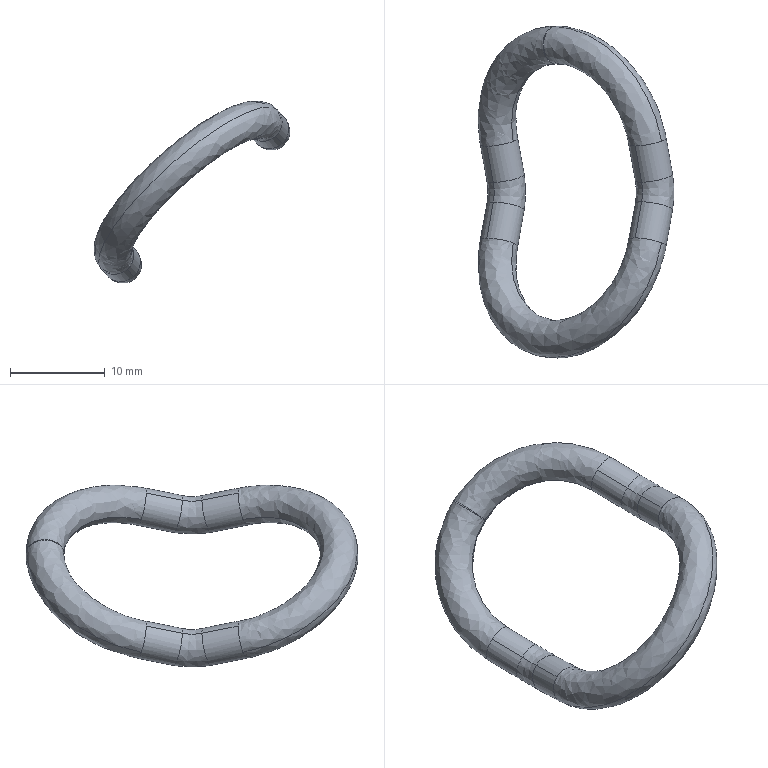Part | SolidWorks | features BaseBody 1 | 1 solid | 20 faces | box 20.665 x 35 x 19.212 mm | volume 1105 mm3 | spline 10 | cylinder 8 | plane 2 | commonest cylinder face diameters 4 x8
STEP:
#1=CARTESIAN_POINT('',(31.371,117.925,197.071));
#2=VERTEX_POINT('',#1);
#3=CARTESIAN_POINT('',(31.572,118.442,199.845));
#4=VERTEX_POINT('',#3);
#5=CARTESIAN_POINT('',(30.082,118.442,198.51));
#6=DIRECTION('',(-0.1727,-0.9659,0.1928));
#7=DIRECTION('',(-0.7448,0.,-0.6673));
#8=AXIS2_PLACEMENT_3D('',#5,#6,#7);
#9=CIRCLE('',#8,2.);
#10=EDGE_CURVE('',#2,#4,#9,.T.);
#11=ORIENTED_EDGE('',*,*,#10,.T.);
#12=CARTESIAN_POINT('',(44.233,118.442,211.189));
#13=VERTEX_POINT('',#12);
#14=CARTESIAN_POINT('',(37.902,118.442,205.517));
#15=DIRECTION('',(-0.6446,0.2588,0.7194));
#16=DIRECTION('',(0.7448,0.,0.6673));
#17=AXIS2_PLACEMENT_3D('',#14,#15,#16);
#18=CIRCLE('',#17,8.5);
#19=EDGE_CURVE('',#4,#13,#18,.T.);
#20=ORIENTED_EDGE('',*,*,#19,.T.);
#21=CARTESIAN_POINT('',(47.012,117.925,211.085));
#22=VERTEX_POINT('',#21);
#23=CARTESIAN_POINT('',(45.723,118.442,212.524));
#24=DIRECTION('',(-0.1727,-0.9659,0.1928));
#25=DIRECTION('',(0.7448,0.,0.6673));
#26=AXIS2_PLACEMENT_3D('',#23,#24,#25);
#27=CIRCLE('',#26,2.);
#28=EDGE_CURVE('',#13,#22,#27,.T.);
#29=ORIENTED_EDGE('',*,*,#28,.T.);
#30=CARTESIAN_POINT('',(47.212,118.442,213.858));
#31=VERTEX_POINT('',#30);
#32=CARTESIAN_POINT('',(45.723,118.442,212.524));
#33=DIRECTION('',(-0.1727,-0.9659,0.1928));
#34=DIRECTION('',(0.7448,0.,0.6673));
#35=AXIS2_PLACEMENT_3D('',#32,#33,#34);
#36=CIRCLE('',#35,2.);
#37=EDGE_CURVE('',#22,#31,#36,.T.);
#38=ORIENTED_EDGE('',*,*,#37,.T.);
#39=CARTESIAN_POINT('',(28.593,118.442,197.176));
#40=VERTEX_POINT('',#39);
#41=CARTESIAN_POINT('',(37.902,118.442,205.517));
#42=DIRECTION('',(-0.6446,0.2588,0.7194));
#43=DIRECTION('',(0.7448,0.,0.6673));
#44=AXIS2_PLACEMENT_3D('',#41,#42,#43);
#45=CIRCLE('',#44,12.5);
#46=EDGE_CURVE('',#40,#31,#45,.T.);
#47=ORIENTED_EDGE('',*,*,#46,.F.);
#48=CARTESIAN_POINT('',(30.082,118.442,198.51));
#49=DIRECTION('',(-0.1727,-0.9659,0.1928));
#50=DIRECTION('',(-0.7448,0.,-0.6673));
#51=AXIS2_PLACEMENT_3D('',#48,#49,#50);
#52=CIRCLE('',#51,2.);
#53=EDGE_CURVE('',#40,#2,#52,.T.);
#54=ORIENTED_EDGE('',*,*,#53,.T.);
#55=EDGE_LOOP('',(#11,#20,#29,#38,#47,#54));
#56=FACE_OUTER_BOUND('',#55,.T.);
#57=CARTESIAN_POINT('',(28.593,118.442,197.176));
#58=CARTESIAN_POINT('',(24.275,94.294,201.995));
#59=CARTESIAN_POINT('',(42.894,94.294,218.677));
#60=CARTESIAN_POINT('',(47.212,118.442,213.858));
#61=CARTESIAN_POINT('',(31.171,117.407,194.298));
#62=CARTESIAN_POINT('',(26.853,93.259,199.117));
#63=CARTESIAN_POINT('',(45.473,93.259,215.8));
#64=CARTESIAN_POINT('',(49.79,117.407,210.981));
#65=CARTESIAN_POINT('',(34.15,117.407,196.967));
#66=CARTESIAN_POINT('',(31.214,100.986,200.244));
#67=CARTESIAN_POINT('',(43.875,100.986,211.588));
#68=CARTESIAN_POINT('',(46.811,117.407,208.311));
#69=CARTESIAN_POINT('',(31.572,118.442,199.845));
#70=CARTESIAN_POINT('',(28.636,102.021,203.122));
#71=CARTESIAN_POINT('',(41.297,102.021,214.466));
#72=CARTESIAN_POINT('',(44.233,118.442,211.189));
#73=(BOUNDED_SURFACE()B_SPLINE_SURFACE(3,3,((#57,#58,#59,#60),(#61,#62,#63,#64),(#65,#66,#67,#68),(#69,#70,#71,#72)),.UNSPECIFIED.,.F.,.F.,.T.)B_SPLINE_SURFACE_WITH_KNOTS((4,4),(4,4),(0.,1.),(0.,1.),.UNSPECIFIED.)GEOMETRIC_REPRESENTATION_ITEM()RATIONAL_B_SPLINE_SURFACE(((1.,0.3333,0.3333,1.),(0.3333,0.1111,0.1111,0.3333),(0.3333,0.1111,0.1111,0.3333),(1.,0.3333,0.3333,1.)))REPRESENTATION_ITEM('')SURFACE());
#74=ADVANCED_FACE('',(#56),#73,.T.);
#75=CARTESIAN_POINT('',(29.473,122.765,199.19));
#76=VERTEX_POINT('',#75);
#77=CARTESIAN_POINT('',(32.052,121.729,196.312));
#78=VERTEX_POINT('',#77);
#79=CARTESIAN_POINT('',(30.763,122.247,197.751));
#80=DIRECTION('',(-0.1727,-0.9659,0.1928));
#81=DIRECTION('',(-0.6446,0.2588,0.7194));
#82=AXIS2_PLACEMENT_3D('',#79,#80,#81);
#83=CIRCLE('',#82,2.);
#84=EDGE_CURVE('',#76,#78,#83,.T.);
#85=ORIENTED_EDGE('',*,*,#84,.T.);
#86=CARTESIAN_POINT('',(32.052,121.729,196.312));
#87=DIRECTION('',(-0.1727,-0.9659,0.1928));
#88=VECTOR('',#87,1000.);
#89=LINE('',#86,#88);
#90=EDGE_CURVE('',#78,#2,#89,.T.);
#91=ORIENTED_EDGE('',*,*,#90,.T.);
#92=ORIENTED_EDGE('',*,*,#53,.F.);
#93=CARTESIAN_POINT('',(28.793,118.96,199.949));
#94=VERTEX_POINT('',#93);
#95=CARTESIAN_POINT('',(30.082,118.442,198.51));
#96=DIRECTION('',(-0.1727,-0.9659,0.1928));
#97=DIRECTION('',(-0.7448,0.,-0.6673));
#98=AXIS2_PLACEMENT_3D('',#95,#96,#97);
#99=CIRCLE('',#98,2.);
#100=EDGE_CURVE('',#94,#40,#99,.T.);
#101=ORIENTED_EDGE('',*,*,#100,.F.);
#102=CARTESIAN_POINT('',(29.473,122.765,199.19));
#103=DIRECTION('',(-0.1727,-0.9659,0.1928));
#104=VECTOR('',#103,1000.);
#105=LINE('',#102,#104);
#106=EDGE_CURVE('',#76,#94,#105,.T.);
#107=ORIENTED_EDGE('',*,*,#106,.F.);
#108=EDGE_LOOP('',(#85,#91,#92,#101,#107));
#109=FACE_OUTER_BOUND('',#108,.T.);
#110=CARTESIAN_POINT('',(30.763,122.247,197.751));
#111=DIRECTION('',(-0.1727,-0.9659,0.1928));
#112=DIRECTION('',(-0.6446,0.2588,0.7194));
#113=AXIS2_PLACEMENT_3D('',#110,#111,#112);
#114=CYLINDRICAL_SURFACE('',#113,2.);
#115=ADVANCED_FACE('',(#109),#114,.T.);
#116=CARTESIAN_POINT('',(44.433,118.96,213.963));
#117=VERTEX_POINT('',#116);
#118=CARTESIAN_POINT('',(45.723,118.442,212.524));
#119=DIRECTION('',(-0.1727,-0.9659,0.1928));
#120=DIRECTION('',(0.7448,0.,0.6673));
#121=AXIS2_PLACEMENT_3D('',#118,#119,#120);
#122=CIRCLE('',#121,2.);
#123=EDGE_CURVE('',#117,#13,#122,.T.);
#124=ORIENTED_EDGE('',*,*,#123,.F.);
#125=CARTESIAN_POINT('',(45.114,122.765,213.203));
#126=VERTEX_POINT('',#125);
#127=CARTESIAN_POINT('',(44.433,118.96,213.963));
#128=DIRECTION('',(0.1727,0.9659,-0.1928));
#129=VECTOR('',#128,1000.);
#130=LINE('',#127,#129);
#131=EDGE_CURVE('',#117,#126,#130,.T.);
#132=ORIENTED_EDGE('',*,*,#131,.T.);
#133=CARTESIAN_POINT('',(47.692,121.729,210.326));
#134=VERTEX_POINT('',#133);
#135=CARTESIAN_POINT('',(46.403,122.247,211.764));
#136=DIRECTION('',(-0.1727,-0.9659,0.1928));
#137=DIRECTION('',(0.6446,-0.2588,-0.7194));
#138=AXIS2_PLACEMENT_3D('',#135,#136,#137);
#139=CIRCLE('',#138,2.);
#140=EDGE_CURVE('',#126,#134,#139,.T.);
#141=ORIENTED_EDGE('',*,*,#140,.T.);
#142=CARTESIAN_POINT('',(47.012,117.925,211.085));
#143=DIRECTION('',(0.1727,0.9659,-0.1928));
#144=VECTOR('',#143,1000.);
#145=LINE('',#142,#144);
#146=EDGE_CURVE('',#22,#134,#145,.T.);
#147=ORIENTED_EDGE('',*,*,#146,.F.);
#148=ORIENTED_EDGE('',*,*,#28,.F.);
#149=EDGE_LOOP('',(#124,#132,#141,#147,#148));
#150=FACE_OUTER_BOUND('',#149,.T.);
#151=CARTESIAN_POINT('',(45.723,118.442,212.524));
#152=DIRECTION('',(0.1727,0.9659,-0.1928));
#153=DIRECTION('',(0.6446,-0.2588,-0.7194));
#154=AXIS2_PLACEMENT_3D('',#151,#152,#153);
#155=CYLINDRICAL_SURFACE('',#154,2.);
#156=ADVANCED_FACE('',(#150),#155,.T.);
#157=CARTESIAN_POINT('',(32.052,125.871,196.312));
#158=VERTEX_POINT('',#157);
#159=CARTESIAN_POINT('',(29.473,124.835,199.19));
#160=VERTEX_POINT('',#159);
#161=CARTESIAN_POINT('',(30.763,125.353,197.751));
#162=DIRECTION('',(0.1727,-0.9659,-0.1928));
#163=DIRECTION('',(0.6446,0.2588,-0.7194));
#164=AXIS2_PLACEMENT_3D('',#161,#162,#163);
#165=CIRCLE('',#164,2.);
#166=EDGE_CURVE('',#158,#160,#165,.T.);
#167=ORIENTED_EDGE('',*,*,#166,.T.);
#168=CARTESIAN_POINT('',(26.895,123.8,202.067));
#169=DIRECTION('',(-0.7448,0.,-0.6673));
#170=DIRECTION('',(-0.6446,-0.2588,0.7194));
#171=AXIS2_PLACEMENT_3D('',#168,#169,#170);
#172=CIRCLE('',#171,4.);
#173=EDGE_CURVE('',#160,#76,#172,.T.);
#174=ORIENTED_EDGE('',*,*,#173,.T.);
#175=CARTESIAN_POINT('',(30.763,122.247,197.751));
#176=DIRECTION('',(-0.1727,-0.9659,0.1928));
#177=DIRECTION('',(-0.6446,0.2588,0.7194));
#178=AXIS2_PLACEMENT_3D('',#175,#176,#177);
#179=CIRCLE('',#178,2.);
#180=EDGE_CURVE('',#78,#76,#179,.T.);
#181=ORIENTED_EDGE('',*,*,#180,.F.);
#182=CARTESIAN_POINT('',(26.895,123.8,202.067));
#183=DIRECTION('',(-0.7448,0.,-0.6673));
#184=DIRECTION('',(-0.6446,-0.2588,0.7194));
#185=AXIS2_PLACEMENT_3D('',#182,#183,#184);
#186=CIRCLE('',#185,8.);
#187=EDGE_CURVE('',#158,#78,#186,.T.);
#188=ORIENTED_EDGE('',*,*,#187,.F.);
#189=EDGE_LOOP('',(#167,#174,#181,#188));
#190=FACE_OUTER_BOUND('',#189,.T.);
#191=CARTESIAN_POINT('',(32.052,125.871,196.312));
#192=CARTESIAN_POINT('',(32.296,124.506,196.04));
#193=CARTESIAN_POINT('',(32.296,123.094,196.04));
#194=CARTESIAN_POINT('',(32.052,121.729,196.312));
#195=CARTESIAN_POINT('',(35.031,125.871,198.981));
#196=CARTESIAN_POINT('',(35.275,124.506,198.709));
#197=CARTESIAN_POINT('',(35.275,123.094,198.709));
#198=CARTESIAN_POINT('',(35.031,121.729,198.981));
#199=CARTESIAN_POINT('',(32.453,124.835,201.859));
#200=CARTESIAN_POINT('',(32.574,124.153,201.723));
#201=CARTESIAN_POINT('',(32.574,123.447,201.723));
#202=CARTESIAN_POINT('',(32.453,122.765,201.859));
#203=CARTESIAN_POINT('',(29.473,124.835,199.19));
#204=CARTESIAN_POINT('',(29.595,124.153,199.054));
#205=CARTESIAN_POINT('',(29.595,123.447,199.054));
#206=CARTESIAN_POINT('',(29.473,122.765,199.19));
#207=(BOUNDED_SURFACE()B_SPLINE_SURFACE(3,3,((#191,#192,#193,#194),(#195,#196,#197,#198),(#199,#200,#201,#202),(#203,#204,#205,#206)),.UNSPECIFIED.,.F.,.F.,.F.)B_SPLINE_SURFACE_WITH_KNOTS((4,4),(4,4),(0.,1.),(0.,1.),.UNSPECIFIED.)GEOMETRIC_REPRESENTATION_ITEM()RATIONAL_B_SPLINE_SURFACE(((1.,0.9773,0.9773,1.),(0.3333,0.3258,0.3258,0.3333),(0.3333,0.3258,0.3258,0.3333),(1.,0.9773,0.9773,1.)))REPRESENTATION_ITEM('')SURFACE());
#208=ADVANCED_FACE('',(#190),#207,.T.);
#209=ORIENTED_EDGE('',*,*,#140,.F.);
#210=CARTESIAN_POINT('',(45.114,124.835,213.203));
#211=VERTEX_POINT('',#210);
#212=CARTESIAN_POINT('',(42.535,123.8,216.081));
#213=DIRECTION('',(0.7448,0.,0.6673));
#214=DIRECTION('',(-0.6446,0.2588,0.7194));
#215=AXIS2_PLACEMENT_3D('',#212,#213,#214);
#216=CIRCLE('',#215,4.);
#217=EDGE_CURVE('',#126,#211,#216,.T.);
#218=ORIENTED_EDGE('',*,*,#217,.T.);
#219=CARTESIAN_POINT('',(47.692,125.871,210.326));
#220=VERTEX_POINT('',#219);
#221=CARTESIAN_POINT('',(46.403,125.353,211.764));
#222=DIRECTION('',(0.1727,-0.9659,-0.1928));
#223=DIRECTION('',(0.6446,0.2588,-0.7194));
#224=AXIS2_PLACEMENT_3D('',#221,#222,#223);
#225=CIRCLE('',#224,2.);
#226=EDGE_CURVE('',#211,#220,#225,.T.);
#227=ORIENTED_EDGE('',*,*,#226,.T.);
#228=CARTESIAN_POINT('',(42.535,123.8,216.081));
#229=DIRECTION('',(0.7448,0.,0.6673));
#230=DIRECTION('',(-0.6446,0.2588,0.7194));
#231=AXIS2_PLACEMENT_3D('',#228,#229,#230);
#232=CIRCLE('',#231,8.);
#233=EDGE_CURVE('',#134,#220,#232,.T.);
#234=ORIENTED_EDGE('',*,*,#233,.F.);
#235=EDGE_LOOP('',(#209,#218,#227,#234));
#236=FACE_OUTER_BOUND('',#235,.T.);
#237=CARTESIAN_POINT('',(47.692,121.729,210.326));
#238=CARTESIAN_POINT('',(47.936,123.094,210.053));
#239=CARTESIAN_POINT('',(47.936,124.506,210.053));
#240=CARTESIAN_POINT('',(47.692,125.871,210.326));
#241=CARTESIAN_POINT('',(44.713,121.729,207.656));
#242=CARTESIAN_POINT('',(44.957,123.094,207.384));
#243=CARTESIAN_POINT('',(44.957,124.506,207.384));
#244=CARTESIAN_POINT('',(44.713,125.871,207.656));
#245=CARTESIAN_POINT('',(42.135,122.765,210.534));
#246=CARTESIAN_POINT('',(42.257,123.447,210.398));
#247=CARTESIAN_POINT('',(42.257,124.153,210.398));
#248=CARTESIAN_POINT('',(42.135,124.835,210.534));
#249=CARTESIAN_POINT('',(45.114,122.765,213.203));
#250=CARTESIAN_POINT('',(45.236,123.447,213.067));
#251=CARTESIAN_POINT('',(45.236,124.153,213.067));
#252=CARTESIAN_POINT('',(45.114,124.835,213.203));
#253=(BOUNDED_SURFACE()B_SPLINE_SURFACE(3,3,((#237,#238,#239,#240),(#241,#242,#243,#244),(#245,#246,#247,#248),(#249,#250,#251,#252)),.UNSPECIFIED.,.F.,.F.,.T.)B_SPLINE_SURFACE_WITH_KNOTS((4,4),(4,4),(0.,1.),(0.,1.),.UNSPECIFIED.)GEOMETRIC_REPRESENTATION_ITEM()RATIONAL_B_SPLINE_SURFACE(((1.,0.9773,0.9773,1.),(0.3333,0.3258,0.3258,0.3333),(0.3333,0.3258,0.3258,0.3333),(1.,0.9773,0.9773,1.)))REPRESENTATION_ITEM('')SURFACE());
#254=ADVANCED_FACE('',(#236),#253,.T.);
#255=CARTESIAN_POINT('',(28.593,129.158,197.176));
#256=VERTEX_POINT('',#255);
#257=CARTESIAN_POINT('',(31.371,129.675,197.071));
#258=VERTEX_POINT('',#257);
#259=CARTESIAN_POINT('',(30.082,129.158,198.51));
#260=DIRECTION('',(0.1727,-0.9659,-0.1928));
#261=DIRECTION('',(-0.6446,-0.2588,0.7194));
#262=AXIS2_PLACEMENT_3D('',#259,#260,#261);
#263=CIRCLE('',#262,2.);
#264=EDGE_CURVE('',#256,#258,#263,.T.);
#265=ORIENTED_EDGE('',*,*,#264,.T.);
#266=CARTESIAN_POINT('',(31.371,129.675,197.071));
#267=DIRECTION('',(0.1727,-0.9659,-0.1928));
#268=VECTOR('',#267,1000.);
#269=LINE('',#266,#268);
#270=EDGE_CURVE('',#258,#158,#269,.T.);
#271=ORIENTED_EDGE('',*,*,#270,.T.);
#272=CARTESIAN_POINT('',(30.763,125.353,197.751));
#273=DIRECTION('',(0.1727,-0.9659,-0.1928));
#274=DIRECTION('',(0.6446,0.2588,-0.7194));
#275=AXIS2_PLACEMENT_3D('',#272,#273,#274);
#276=CIRCLE('',#275,2.);
#277=EDGE_CURVE('',#160,#158,#276,.T.);
#278=ORIENTED_EDGE('',*,*,#277,.F.);
#279=CARTESIAN_POINT('',(28.793,128.64,199.949));
#280=VERTEX_POINT('',#279);
#281=CARTESIAN_POINT('',(28.793,128.64,199.949));
#282=DIRECTION('',(0.1727,-0.9659,-0.1928));
#283=VECTOR('',#282,1000.);
#284=LINE('',#281,#283);
#285=EDGE_CURVE('',#280,#160,#284,.T.);
#286=ORIENTED_EDGE('',*,*,#285,.F.);
#287=CARTESIAN_POINT('',(30.082,129.158,198.51));
#288=DIRECTION('',(0.1727,-0.9659,-0.1928));
#289=DIRECTION('',(-0.6446,-0.2588,0.7194));
#290=AXIS2_PLACEMENT_3D('',#287,#288,#289);
#291=CIRCLE('',#290,2.);
#292=EDGE_CURVE('',#280,#256,#291,.T.);
#293=ORIENTED_EDGE('',*,*,#292,.T.);
#294=EDGE_LOOP('',(#265,#271,#278,#286,#293));
#295=FACE_OUTER_BOUND('',#294,.T.);
#296=CARTESIAN_POINT('',(30.082,129.158,198.51));
#297=DIRECTION('',(0.1727,-0.9659,-0.1928));
#298=DIRECTION('',(-0.6446,-0.2588,0.7194));
#299=AXIS2_PLACEMENT_3D('',#296,#297,#298);
#300=CYLINDRICAL_SURFACE('',#299,2.);
#301=ADVANCED_FACE('',(#295),#300,.T.);
#302=ORIENTED_EDGE('',*,*,#226,.F.);
#303=CARTESIAN_POINT('',(44.433,128.64,213.963));
#304=VERTEX_POINT('',#303);
#305=CARTESIAN_POINT('',(45.114,124.835,213.203));
#306=DIRECTION('',(-0.1727,0.9659,0.1928));
#307=VECTOR('',#306,1000.);
#308=LINE('',#305,#307);
#309=EDGE_CURVE('',#211,#304,#308,.T.);
#310=ORIENTED_EDGE('',*,*,#309,.T.);
#311=CARTESIAN_POINT('',(44.233,129.158,211.189));
#312=VERTEX_POINT('',#311);
#313=CARTESIAN_POINT('',(45.723,129.158,212.524));
#314=DIRECTION('',(0.1727,-0.9659,-0.1928));
#315=DIRECTION('',(0.6446,0.2588,-0.7194));
#316=AXIS2_PLACEMENT_3D('',#313,#314,#315);
#317=CIRCLE('',#316,2.);
#318=EDGE_CURVE('',#304,#312,#317,.T.);
#319=ORIENTED_EDGE('',*,*,#318,.T.);
#320=CARTESIAN_POINT('',(47.012,129.675,211.085));
#321=VERTEX_POINT('',#320);
#322=CARTESIAN_POINT('',(45.723,129.158,212.524));
#323=DIRECTION('',(0.1727,-0.9659,-0.1928));
#324=DIRECTION('',(0.6446,0.2588,-0.7194));
#325=AXIS2_PLACEMENT_3D('',#322,#323,#324);
#326=CIRCLE('',#325,2.);
#327=EDGE_CURVE('',#312,#321,#326,.T.);
#328=ORIENTED_EDGE('',*,*,#327,.T.);
#329=CARTESIAN_POINT('',(47.692,125.871,210.326));
#330=DIRECTION('',(-0.1727,0.9659,0.1928));
#331=VECTOR('',#330,1000.);
#332=LINE('',#329,#331);
#333=EDGE_CURVE('',#220,#321,#332,.T.);
#334=ORIENTED_EDGE('',*,*,#333,.F.);
#335=EDGE_LOOP('',(#302,#310,#319,#328,#334));
#336=FACE_OUTER_BOUND('',#335,.T.);
#337=CARTESIAN_POINT('',(46.403,125.353,211.764));
#338=DIRECTION('',(-0.1727,0.9659,0.1928));
#339=DIRECTION('',(0.6446,0.2588,-0.7194));
#340=AXIS2_PLACEMENT_3D('',#337,#338,#339);
#341=CYLINDRICAL_SURFACE('',#340,2.);
#342=ADVANCED_FACE('',(#336),#341,.T.);
#343=CARTESIAN_POINT('',(35.706,141.232,207.893));
#344=VERTEX_POINT('',#343);
#345=CARTESIAN_POINT('',(36.397,137.368,207.122));
#346=VERTEX_POINT('',#345);
#347=CARTESIAN_POINT('',(35.706,141.232,207.893));
#348=CARTESIAN_POINT('',(35.831,141.282,207.754));
#349=CARTESIAN_POINT('',(35.975,141.311,207.593));
#350=CARTESIAN_POINT('',(36.29,141.282,207.241));
#351=CARTESIAN_POINT('',(36.462,141.223,207.049));
#352=CARTESIAN_POINT('',(36.793,140.985,206.679));
#353=CARTESIAN_POINT('',(36.951,140.806,206.503));
#354=CARTESIAN_POINT('',(37.139,140.469,206.294));
#355=CARTESIAN_POINT('',(37.193,140.346,206.233));
#356=CARTESIAN_POINT('',(37.26,140.153,206.159));
#357=CARTESIAN_POINT('',(37.279,140.087,206.137));
#358=CARTESIAN_POINT('',(37.305,139.987,206.108));
#359=CARTESIAN_POINT('',(37.317,139.937,206.095));
#360=CARTESIAN_POINT('',(37.329,139.878,206.081));
#361=CARTESIAN_POINT('',(37.335,139.848,206.075));
#362=CARTESIAN_POINT('',(37.338,139.836,206.072));
#363=CARTESIAN_POINT('',(37.339,139.827,206.071));
#364=CARTESIAN_POINT('',(37.339,139.825,206.07));
#365=CARTESIAN_POINT('',(37.376,139.62,206.029));
#366=CARTESIAN_POINT('',(37.39,139.418,206.014));
#367=CARTESIAN_POINT('',(37.381,139.034,206.025));
#368=CARTESIAN_POINT('',(37.358,138.853,206.05));
#369=CARTESIAN_POINT('',(37.288,138.526,206.128));
#370=CARTESIAN_POINT('',(37.242,138.381,206.18));
#371=CARTESIAN_POINT('',(37.138,138.127,206.297));
#372=CARTESIAN_POINT('',(37.08,138.018,206.361));
#373=CARTESIAN_POINT('',(36.906,137.741,206.556));
#374=CARTESIAN_POINT('',(36.787,137.62,206.688));
#375=CARTESIAN_POINT('',(36.574,137.451,206.925));
#376=CARTESIAN_POINT('',(36.479,137.401,207.03));
#377=CARTESIAN_POINT('',(36.397,137.368,207.122));
#378=B_SPLINE_CURVE_WITH_KNOTS('',3,(#347,#348,#349,#350,#351,#352,#353,#354,#355,#356,#357,#358,#359,#360,#361,#362,#363,#364,#365,#366,#367,#368,#369,#370,#371,#372,#373,#374,#375,#376,#377),.UNSPECIFIED.,.F.,.F.,(4,2,2,2,2,2,1,1,1,2,2,2,2,2,2,2,4),(0.,0.125,0.25,0.375,0.4375,0.4687,0.4844,0.4922,0.4961,0.498,0.5,0.5625,0.625,0.6875,0.75,0.875,1.),.UNSPECIFIED.);
#379=EDGE_CURVE('',#344,#346,#378,.T.);
#380=ORIENTED_EDGE('',*,*,#379,.T.);
#381=CARTESIAN_POINT('',(31.572,129.158,199.845));
#382=VERTEX_POINT('',#381);
#383=CARTESIAN_POINT('',(37.902,129.158,205.517));
#384=DIRECTION('',(-0.6446,-0.2588,0.7194));
#385=DIRECTION('',(-0.7448,0.,-0.6673));
#386=AXIS2_PLACEMENT_3D('',#383,#384,#385);
#387=CIRCLE('',#386,8.5);
#388=EDGE_CURVE('',#346,#382,#387,.T.);
#389=ORIENTED_EDGE('',*,*,#388,.T.);
#390=CARTESIAN_POINT('',(30.082,129.158,198.51));
#391=DIRECTION('',(0.1727,-0.9659,-0.1928));
#392=DIRECTION('',(-0.6446,-0.2588,0.7194));
#393=AXIS2_PLACEMENT_3D('',#390,#391,#392);
#394=CIRCLE('',#393,2.);
#395=EDGE_CURVE('',#258,#382,#394,.T.);
#396=ORIENTED_EDGE('',*,*,#395,.F.);
#397=ORIENTED_EDGE('',*,*,#264,.F.);
#398=CARTESIAN_POINT('',(37.902,129.158,205.517));
#399=DIRECTION('',(-0.6446,-0.2588,0.7194));
#400=DIRECTION('',(-0.7448,0.,-0.6673));
#401=AXIS2_PLACEMENT_3D('',#398,#399,#400);
#402=CIRCLE('',#401,12.5);
#403=EDGE_CURVE('',#344,#256,#402,.T.);
#404=ORIENTED_EDGE('',*,*,#403,.F.);
#405=EDGE_LOOP('',(#380,#389,#396,#397,#404));
#406=FACE_OUTER_BOUND('',#405,.T.);
#407=CARTESIAN_POINT('',(35.794,141.232,207.971));
#408=CARTESIAN_POINT('',(30.31,141.27,203.072));
#409=CARTESIAN_POINT('',(27.323,136.261,198.593));
#410=CARTESIAN_POINT('',(28.593,129.158,197.176));
#411=CARTESIAN_POINT('',(38.372,142.267,205.094));
#412=CARTESIAN_POINT('',(32.888,142.305,200.194));
#413=CARTESIAN_POINT('',(29.901,137.296,195.715));
#414=CARTESIAN_POINT('',(31.171,130.193,194.298));
#415=CARTESIAN_POINT('',(39.047,138.403,204.308));
#416=CARTESIAN_POINT('',(35.318,138.429,200.977));
#417=CARTESIAN_POINT('',(33.286,135.023,197.931));
#418=CARTESIAN_POINT('',(34.15,130.193,196.967));
#419=CARTESIAN_POINT('',(36.469,137.368,207.186));
#420=CARTESIAN_POINT('',(32.74,137.394,203.854));
#421=CARTESIAN_POINT('',(30.708,133.988,200.809));
#422=CARTESIAN_POINT('',(31.572,129.158,199.845));
#423=(BOUNDED_SURFACE()B_SPLINE_SURFACE(3,3,((#407,#408,#409,#410),(#411,#412,#413,#414),(#415,#416,#417,#418),(#419,#420,#421,#422)),.UNSPECIFIED.,.F.,.F.,.T.)B_SPLINE_SURFACE_WITH_KNOTS((4,4),(4,4),(0.,1.),(0.,1.),.UNSPECIFIED.)GEOMETRIC_REPRESENTATION_ITEM()RATIONAL_B_SPLINE_SURFACE(((1.,0.8035,0.8035,1.),(0.3333,0.2678,0.2678,0.3333),(0.3333,0.2678,0.2678,0.3333),(1.,0.8035,0.8035,1.)))REPRESENTATION_ITEM('')SURFACE());
#424=ADVANCED_FACE('',(#406),#423,.T.);
#425=ORIENTED_EDGE('',*,*,#327,.F.);
#426=CARTESIAN_POINT('',(36.472,137.368,207.189));
#427=VERTEX_POINT('',#426);
#428=CARTESIAN_POINT('',(37.902,129.158,205.517));
#429=DIRECTION('',(-0.6446,-0.2588,0.7194));
#430=DIRECTION('',(-0.7448,0.,-0.6673));
#431=AXIS2_PLACEMENT_3D('',#428,#429,#430);
#432=CIRCLE('',#431,8.5);
#433=EDGE_CURVE('',#312,#427,#432,.T.);
#434=ORIENTED_EDGE('',*,*,#433,.T.);
#435=CARTESIAN_POINT('',(35.781,141.232,207.96));
#436=VERTEX_POINT('',#435);
#437=CARTESIAN_POINT('',(36.472,137.368,207.189));
#438=CARTESIAN_POINT('',(36.554,137.401,207.097));
#439=CARTESIAN_POINT('',(36.648,137.451,206.991));
#440=CARTESIAN_POINT('',(36.861,137.621,206.754));
#441=CARTESIAN_POINT('',(36.979,137.741,206.621));
#442=CARTESIAN_POINT('',(37.154,138.018,206.426));
#443=CARTESIAN_POINT('',(37.211,138.127,206.362));
#444=CARTESIAN_POINT('',(37.315,138.38,206.246));
#445=CARTESIAN_POINT('',(37.362,138.526,206.194));
#446=CARTESIAN_POINT('',(37.432,138.852,206.117));
#447=CARTESIAN_POINT('',(37.455,139.033,206.091));
#448=CARTESIAN_POINT('',(37.462,139.32,206.083));
#449=CARTESIAN_POINT('',(37.46,139.418,206.085));
#450=CARTESIAN_POINT('',(37.449,139.567,206.098));
#451=CARTESIAN_POINT('',(37.444,139.617,206.103));
#452=CARTESIAN_POINT('',(37.435,139.692,206.113));
#453=CARTESIAN_POINT('',(37.43,139.729,206.119));
#454=CARTESIAN_POINT('',(37.423,139.773,206.127));
#455=CARTESIAN_POINT('',(37.42,139.791,206.13));
#456=CARTESIAN_POINT('',(37.418,139.804,206.133));
#457=CARTESIAN_POINT('',(37.416,139.812,206.134));
#458=CARTESIAN_POINT('',(37.367,140.087,206.189));
#459=CARTESIAN_POINT('',(37.277,140.355,206.29));
#460=CARTESIAN_POINT('',(37.027,140.805,206.569));
#461=CARTESIAN_POINT('',(36.869,140.985,206.746));
#462=CARTESIAN_POINT('',(36.538,141.222,207.116));
#463=CARTESIAN_POINT('',(36.366,141.282,207.307));
#464=CARTESIAN_POINT('',(36.05,141.311,207.66));
#465=CARTESIAN_POINT('',(35.905,141.282,207.821));
#466=CARTESIAN_POINT('',(35.781,141.232,207.96));
#467=B_SPLINE_CURVE_WITH_KNOTS('',3,(#437,#438,#439,#440,#441,#442,#443,#444,#445,#446,#447,#448,#449,#450,#451,#452,#453,#454,#455,#456,#457,#458,#459,#460,#461,#462,#463,#464,#465,#466),.UNSPECIFIED.,.F.,.F.,(4,2,2,2,2,2,2,2,1,1,2,2,2,2,2,4),(0.,0.125,0.25,0.3125,0.375,0.4375,0.4688,0.4844,0.4922,0.4961,0.498,0.5,0.625,0.75,0.875,1.),.UNSPECIFIED.);
#468=EDGE_CURVE('',#427,#436,#467,.T.);
#469=ORIENTED_EDGE('',*,*,#468,.T.);
#470=CARTESIAN_POINT('',(47.212,129.158,213.858));
#471=VERTEX_POINT('',#470);
#472=CARTESIAN_POINT('',(37.902,129.158,205.517));
#473=DIRECTION('',(-0.6446,-0.2588,0.7194));
#474=DIRECTION('',(-0.7448,0.,-0.6673));
#475=AXIS2_PLACEMENT_3D('',#472,#473,#474);
#476=CIRCLE('',#475,12.5);
#477=EDGE_CURVE('',#471,#436,#476,.T.);
#478=ORIENTED_EDGE('',*,*,#477,.F.);
#479=CARTESIAN_POINT('',(45.723,129.158,212.524));
#480=DIRECTION('',(0.1727,-0.9659,-0.1928));
#481=DIRECTION('',(0.6446,0.2588,-0.7194));
#482=AXIS2_PLACEMENT_3D('',#479,#480,#481);
#483=CIRCLE('',#482,2.);
#484=EDGE_CURVE('',#321,#471,#483,.T.);
#485=ORIENTED_EDGE('',*,*,#484,.F.);
#486=EDGE_LOOP('',(#425,#434,#469,#478,#485));
#487=FACE_OUTER_BOUND('',#486,.T.);
#488=CARTESIAN_POINT('',(47.212,129.158,213.858));
#489=CARTESIAN_POINT('',(45.942,136.261,215.276));
#490=CARTESIAN_POINT('',(41.163,141.27,212.796));
#491=CARTESIAN_POINT('',(35.693,141.232,207.881));
#492=CARTESIAN_POINT('',(49.79,130.193,210.981));
#493=CARTESIAN_POINT('',(48.52,137.296,212.398));
#494=CARTESIAN_POINT('',(43.741,142.305,209.919));
#495=CARTESIAN_POINT('',(38.272,142.267,205.004));
#496=CARTESIAN_POINT('',(46.811,130.193,208.311));
#497=CARTESIAN_POINT('',(45.948,135.023,209.275));
#498=CARTESIAN_POINT('',(42.698,138.429,207.589));
#499=CARTESIAN_POINT('',(38.978,138.403,204.247));
#500=CARTESIAN_POINT('',(44.233,129.158,211.189));
#501=CARTESIAN_POINT('',(43.369,133.988,212.153));
#502=CARTESIAN_POINT('',(40.12,137.394,210.467));
#503=CARTESIAN_POINT('',(36.4,137.368,207.125));
#504=(BOUNDED_SURFACE()B_SPLINE_SURFACE(3,3,((#488,#489,#490,#491),(#492,#493,#494,#495),(#496,#497,#498,#499),(#500,#501,#502,#503)),.UNSPECIFIED.,.F.,.F.,.T.)B_SPLINE_SURFACE_WITH_KNOTS((4,4),(4,4),(0.,1.),(0.,1.),.UNSPECIFIED.)GEOMETRIC_REPRESENTATION_ITEM()RATIONAL_B_SPLINE_SURFACE(((1.,0.8035,0.8035,1.),(0.3333,0.2678,0.2678,0.3333),(0.3333,0.2678,0.2678,0.3333),(1.,0.8035,0.8035,1.)))REPRESENTATION_ITEM('')SURFACE());
#505=ADVANCED_FACE('',(#487),#504,.T.);
#506=ORIENTED_EDGE('',*,*,#19,.F.);
#507=CARTESIAN_POINT('',(30.082,118.442,198.51));
#508=DIRECTION('',(-0.1727,-0.9659,0.1928));
#509=DIRECTION('',(-0.7448,0.,-0.6673));
#510=AXIS2_PLACEMENT_3D('',#507,#508,#509);
#511=CIRCLE('',#510,2.);
#512=EDGE_CURVE('',#4,#94,#511,.T.);
#513=ORIENTED_EDGE('',*,*,#512,.T.);
#514=ORIENTED_EDGE('',*,*,#100,.T.);
#515=ORIENTED_EDGE('',*,*,#46,.T.);
#516=CARTESIAN_POINT('',(45.723,118.442,212.524));
#517=DIRECTION('',(-0.1727,-0.9659,0.1928));
#518=DIRECTION('',(0.7448,0.,0.6673));
#519=AXIS2_PLACEMENT_3D('',#516,#517,#518);
#520=CIRCLE('',#519,2.);
#521=EDGE_CURVE('',#31,#117,#520,.T.);
#522=ORIENTED_EDGE('',*,*,#521,.T.);
#523=ORIENTED_EDGE('',*,*,#123,.T.);
#524=EDGE_LOOP('',(#506,#513,#514,#515,#522,#523));
#525=FACE_OUTER_BOUND('',#524,.T.);
#526=CARTESIAN_POINT('',(31.572,118.442,199.845));
#527=CARTESIAN_POINT('',(28.636,102.021,203.122));
#528=CARTESIAN_POINT('',(41.297,102.021,214.466));
#529=CARTESIAN_POINT('',(44.233,118.442,211.189));
#530=CARTESIAN_POINT('',(28.993,119.477,202.722));
#531=CARTESIAN_POINT('',(26.057,103.057,205.999));
#532=CARTESIAN_POINT('',(38.719,103.057,217.344));
#533=CARTESIAN_POINT('',(41.655,119.477,214.067));
#534=CARTESIAN_POINT('',(26.014,119.477,200.053));
#535=CARTESIAN_POINT('',(21.697,95.329,204.872));
#536=CARTESIAN_POINT('',(40.316,95.329,221.555));
#537=CARTESIAN_POINT('',(44.634,119.477,216.736));
#538=CARTESIAN_POINT('',(28.593,118.442,197.176));
#539=CARTESIAN_POINT('',(24.275,94.294,201.995));
#540=CARTESIAN_POINT('',(42.894,94.294,218.677));
#541=CARTESIAN_POINT('',(47.212,118.442,213.858));
#542=(BOUNDED_SURFACE()B_SPLINE_SURFACE(3,3,((#526,#527,#528,#529),(#530,#531,#532,#533),(#534,#535,#536,#537),(#538,#539,#540,#541)),.UNSPECIFIED.,.F.,.F.,.T.)B_SPLINE_SURFACE_WITH_KNOTS((4,4),(4,4),(0.,1.),(0.,1.),.UNSPECIFIED.)GEOMETRIC_REPRESENTATION_ITEM()RATIONAL_B_SPLINE_SURFACE(((1.,0.3333,0.3333,1.),(0.3333,0.1111,0.1111,0.3333),(0.3333,0.1111,0.1111,0.3333),(1.,0.3333,0.3333,1.)))REPRESENTATION_ITEM('')SURFACE());
#543=ADVANCED_FACE('',(#525),#542,.T.);
#544=ORIENTED_EDGE('',*,*,#90,.F.);
#545=ORIENTED_EDGE('',*,*,#180,.T.);
#546=ORIENTED_EDGE('',*,*,#106,.T.);
#547=ORIENTED_EDGE('',*,*,#512,.F.);
#548=ORIENTED_EDGE('',*,*,#10,.F.);
#549=EDGE_LOOP('',(#544,#545,#546,#547,#548));
#550=FACE_OUTER_BOUND('',#549,.T.);
#551=CARTESIAN_POINT('',(30.763,122.247,197.751));
#552=DIRECTION('',(-0.1727,-0.9659,0.1928));
#553=DIRECTION('',(-0.6446,0.2588,0.7194));
#554=AXIS2_PLACEMENT_3D('',#551,#552,#553);
#555=CYLINDRICAL_SURFACE('',#554,2.);
#556=ADVANCED_FACE('',(#550),#555,.T.);
#557=ORIENTED_EDGE('',*,*,#131,.F.);
#558=ORIENTED_EDGE('',*,*,#521,.F.);
#559=ORIENTED_EDGE('',*,*,#37,.F.);
#560=ORIENTED_EDGE('',*,*,#146,.T.);
#561=CARTESIAN_POINT('',(46.403,122.247,211.764));
#562=DIRECTION('',(-0.1727,-0.9659,0.1928));
#563=DIRECTION('',(0.6446,-0.2588,-0.7194));
#564=AXIS2_PLACEMENT_3D('',#561,#562,#563);
#565=CIRCLE('',#564,2.);
#566=EDGE_CURVE('',#134,#126,#565,.T.);
#567=ORIENTED_EDGE('',*,*,#566,.T.);
#568=EDGE_LOOP('',(#557,#558,#559,#560,#567));
#569=FACE_OUTER_BOUND('',#568,.T.);
#570=CARTESIAN_POINT('',(45.723,118.442,212.524));
#571=DIRECTION('',(0.1727,0.9659,-0.1928));
#572=DIRECTION('',(0.6446,-0.2588,-0.7194));
#573=AXIS2_PLACEMENT_3D('',#570,#571,#572);
#574=CYLINDRICAL_SURFACE('',#573,2.);
#575=ADVANCED_FACE('',(#569),#574,.T.);
#576=ORIENTED_EDGE('',*,*,#173,.F.);
#577=ORIENTED_EDGE('',*,*,#277,.T.);
#578=ORIENTED_EDGE('',*,*,#187,.T.);
#579=ORIENTED_EDGE('',*,*,#84,.F.);
#580=EDGE_LOOP('',(#576,#577,#578,#579));
#581=FACE_OUTER_BOUND('',#580,.T.);
#582=CARTESIAN_POINT('',(29.473,124.835,199.19));
#583=CARTESIAN_POINT('',(29.595,124.153,199.054));
#584=CARTESIAN_POINT('',(29.595,123.447,199.054));
#585=CARTESIAN_POINT('',(29.473,122.765,199.19));
#586=CARTESIAN_POINT('',(26.494,124.835,196.52));
#587=CARTESIAN_POINT('',(26.616,124.153,196.384));
#588=CARTESIAN_POINT('',(26.616,123.447,196.384));
#589=CARTESIAN_POINT('',(26.494,122.765,196.52));
#590=CARTESIAN_POINT('',(29.073,125.871,193.643));
#591=CARTESIAN_POINT('',(29.317,124.506,193.371));
#592=CARTESIAN_POINT('',(29.317,123.094,193.371));
#593=CARTESIAN_POINT('',(29.073,121.729,193.643));
#594=CARTESIAN_POINT('',(32.052,125.871,196.312));
#595=CARTESIAN_POINT('',(32.296,124.506,196.04));
#596=CARTESIAN_POINT('',(32.296,123.094,196.04));
#597=CARTESIAN_POINT('',(32.052,121.729,196.312));
#598=(BOUNDED_SURFACE()B_SPLINE_SURFACE(3,3,((#582,#583,#584,#585),(#586,#587,#588,#589),(#590,#591,#592,#593),(#594,#595,#596,#597)),.UNSPECIFIED.,.F.,.F.,.T.)B_SPLINE_SURFACE_WITH_KNOTS((4,4),(4,4),(0.,1.),(0.,1.),.UNSPECIFIED.)GEOMETRIC_REPRESENTATION_ITEM()RATIONAL_B_SPLINE_SURFACE(((1.,0.9773,0.9773,1.),(0.3333,0.3258,0.3258,0.3333),(0.3333,0.3258,0.3258,0.3333),(1.,0.9773,0.9773,1.)))REPRESENTATION_ITEM('')SURFACE());
#599=ADVANCED_FACE('',(#581),#598,.T.);
#600=ORIENTED_EDGE('',*,*,#217,.F.);
#601=ORIENTED_EDGE('',*,*,#566,.F.);
#602=ORIENTED_EDGE('',*,*,#233,.T.);
#603=CARTESIAN_POINT('',(46.403,125.353,211.764));
#604=DIRECTION('',(0.1727,-0.9659,-0.1928));
#605=DIRECTION('',(0.6446,0.2588,-0.7194));
#606=AXIS2_PLACEMENT_3D('',#603,#604,#605);
#607=CIRCLE('',#606,2.);
#608=EDGE_CURVE('',#220,#211,#607,.T.);
#609=ORIENTED_EDGE('',*,*,#608,.T.);
#610=EDGE_LOOP('',(#600,#601,#602,#609));
#611=FACE_OUTER_BOUND('',#610,.T.);
#612=CARTESIAN_POINT('',(45.114,122.765,213.203));
#613=CARTESIAN_POINT('',(45.236,123.447,213.067));
#614=CARTESIAN_POINT('',(45.236,124.153,213.067));
#615=CARTESIAN_POINT('',(45.114,124.835,213.203));
#616=CARTESIAN_POINT('',(48.093,122.765,215.872));
#617=CARTESIAN_POINT('',(48.215,123.447,215.736));
#618=CARTESIAN_POINT('',(48.215,124.153,215.736));
#619=CARTESIAN_POINT('',(48.093,124.835,215.872));
#620=CARTESIAN_POINT('',(50.671,121.729,212.995));
#621=CARTESIAN_POINT('',(50.915,123.094,212.723));
#622=CARTESIAN_POINT('',(50.915,124.506,212.723));
#623=CARTESIAN_POINT('',(50.671,125.871,212.995));
#624=CARTESIAN_POINT('',(47.692,121.729,210.326));
#625=CARTESIAN_POINT('',(47.936,123.094,210.053));
#626=CARTESIAN_POINT('',(47.936,124.506,210.053));
#627=CARTESIAN_POINT('',(47.692,125.871,210.326));
#628=(BOUNDED_SURFACE()B_SPLINE_SURFACE(3,3,((#612,#613,#614,#615),(#616,#617,#618,#619),(#620,#621,#622,#623),(#624,#625,#626,#627)),.UNSPECIFIED.,.F.,.F.,.T.)B_SPLINE_SURFACE_WITH_KNOTS((4,4),(4,4),(0.,1.),(0.,1.),.UNSPECIFIED.)GEOMETRIC_REPRESENTATION_ITEM()RATIONAL_B_SPLINE_SURFACE(((1.,0.9773,0.9773,1.),(0.3333,0.3258,0.3258,0.3333),(0.3333,0.3258,0.3258,0.3333),(1.,0.9773,0.9773,1.)))REPRESENTATION_ITEM('')SURFACE());
#629=ADVANCED_FACE('',(#611),#628,.T.);
#630=ORIENTED_EDGE('',*,*,#270,.F.);
#631=ORIENTED_EDGE('',*,*,#395,.T.);
#632=CARTESIAN_POINT('',(30.082,129.158,198.51));
#633=DIRECTION('',(0.1727,-0.9659,-0.1928));
#634=DIRECTION('',(-0.6446,-0.2588,0.7194));
#635=AXIS2_PLACEMENT_3D('',#632,#633,#634);
#636=CIRCLE('',#635,2.);
#637=EDGE_CURVE('',#382,#280,#636,.T.);
#638=ORIENTED_EDGE('',*,*,#637,.T.);
#639=ORIENTED_EDGE('',*,*,#285,.T.);
#640=ORIENTED_EDGE('',*,*,#166,.F.);
#641=EDGE_LOOP('',(#630,#631,#638,#639,#640));
#642=FACE_OUTER_BOUND('',#641,.T.);
#643=CARTESIAN_POINT('',(30.082,129.158,198.51));
#644=DIRECTION('',(0.1727,-0.9659,-0.1928));
#645=DIRECTION('',(-0.6446,-0.2588,0.7194));
#646=AXIS2_PLACEMENT_3D('',#643,#644,#645);
#647=CYLINDRICAL_SURFACE('',#646,2.);
#648=ADVANCED_FACE('',(#642),#647,.T.);
#649=ORIENTED_EDGE('',*,*,#309,.F.);
#650=ORIENTED_EDGE('',*,*,#608,.F.);
#651=ORIENTED_EDGE('',*,*,#333,.T.);
#652=ORIENTED_EDGE('',*,*,#484,.T.);
#653=CARTESIAN_POINT('',(45.723,129.158,212.524));
#654=DIRECTION('',(0.1727,-0.9659,-0.1928));
#655=DIRECTION('',(0.6446,0.2588,-0.7194));
#656=AXIS2_PLACEMENT_3D('',#653,#654,#655);
#657=CIRCLE('',#656,2.);
#658=EDGE_CURVE('',#471,#304,#657,.T.);
#659=ORIENTED_EDGE('',*,*,#658,.T.);
#660=EDGE_LOOP('',(#649,#650,#651,#652,#659));
#661=FACE_OUTER_BOUND('',#660,.T.);
#662=CARTESIAN_POINT('',(46.403,125.353,211.764));
#663=DIRECTION('',(-0.1727,0.9659,0.1928));
#664=DIRECTION('',(0.6446,0.2588,-0.7194));
#665=AXIS2_PLACEMENT_3D('',#662,#663,#664);
#666=CYLINDRICAL_SURFACE('',#665,2.);
#667=ADVANCED_FACE('',(#661),#666,.T.);
#668=ORIENTED_EDGE('',*,*,#388,.F.);
#669=CARTESIAN_POINT('',(36.397,137.368,207.122));
#670=CARTESIAN_POINT('',(36.315,137.335,207.214));
#671=CARTESIAN_POINT('',(36.216,137.307,207.324));
#672=CARTESIAN_POINT('',(35.976,137.295,207.593));
#673=CARTESIAN_POINT('',(35.833,137.311,207.753));
#674=CARTESIAN_POINT('',(35.59,137.42,208.024));
#675=CARTESIAN_POINT('',(35.504,137.471,208.12));
#676=CARTESIAN_POINT('',(35.329,137.612,208.315));
#677=CARTESIAN_POINT('',(35.24,137.703,208.414));
#678=CARTESIAN_POINT('',(35.071,137.934,208.603));
#679=CARTESIAN_POINT('',(34.99,138.073,208.693));
#680=CARTESIAN_POINT('',(34.888,138.316,208.807));
#681=CARTESIAN_POINT('',(34.857,138.403,208.841));
#682=CARTESIAN_POINT('',(34.817,138.54,208.886));
#683=CARTESIAN_POINT('',(34.804,138.587,208.9));
#684=CARTESIAN_POINT('',(34.787,138.659,208.919));
#685=CARTESIAN_POINT('',(34.779,138.695,208.928));
#686=CARTESIAN_POINT('',(34.771,138.738,208.937));
#687=CARTESIAN_POINT('',(34.767,138.756,208.941));
#688=CARTESIAN_POINT('',(34.765,138.769,208.944));
#689=CARTESIAN_POINT('',(34.764,138.777,208.945));
#690=CARTESIAN_POINT('',(34.714,139.052,209.));
#691=CARTESIAN_POINT('',(34.703,139.352,209.012));
#692=CARTESIAN_POINT('',(34.769,139.928,208.938));
#693=CARTESIAN_POINT('',(34.846,140.203,208.852));
#694=CARTESIAN_POINT('',(35.054,140.657,208.621));
#695=CARTESIAN_POINT('',(35.183,140.837,208.477));
#696=CARTESIAN_POINT('',(35.447,141.099,208.182));
#697=CARTESIAN_POINT('',(35.582,141.182,208.032));
#698=CARTESIAN_POINT('',(35.706,141.232,207.893));
#699=B_SPLINE_CURVE_WITH_KNOTS('',3,(#669,#670,#671,#672,#673,#674,#675,#676,#677,#678,#679,#680,#681,#682,#683,#684,#685,#686,#687,#688,#689,#690,#691,#692,#693,#694,#695,#696,#697,#698),.UNSPECIFIED.,.F.,.F.,(4,2,2,2,2,2,2,2,1,1,2,2,2,2,2,4),(0.,0.125,0.25,0.3125,0.375,0.4375,0.4687,0.4844,0.4922,0.4961,0.498,0.5,0.625,0.75,0.875,1.),.UNSPECIFIED.);
#700=EDGE_CURVE('',#346,#344,#699,.T.);
#701=ORIENTED_EDGE('',*,*,#700,.T.);
#702=ORIENTED_EDGE('',*,*,#403,.T.);
#703=ORIENTED_EDGE('',*,*,#292,.F.);
#704=ORIENTED_EDGE('',*,*,#637,.F.);
#705=EDGE_LOOP('',(#668,#701,#702,#703,#704));
#706=FACE_OUTER_BOUND('',#705,.T.);
#707=CARTESIAN_POINT('',(36.469,137.368,207.186));
#708=CARTESIAN_POINT('',(32.74,137.394,203.854));
#709=CARTESIAN_POINT('',(30.708,133.988,200.809));
#710=CARTESIAN_POINT('',(31.572,129.158,199.845));
#711=CARTESIAN_POINT('',(33.89,136.333,210.064));
#712=CARTESIAN_POINT('',(30.161,136.359,206.732));
#713=CARTESIAN_POINT('',(28.13,132.953,203.686));
#714=CARTESIAN_POINT('',(28.993,128.123,202.722));
#715=CARTESIAN_POINT('',(33.215,140.196,210.849));
#716=CARTESIAN_POINT('',(27.732,140.235,205.95));
#717=CARTESIAN_POINT('',(24.744,135.226,201.471));
#718=CARTESIAN_POINT('',(26.014,128.123,200.053));
#719=CARTESIAN_POINT('',(35.794,141.232,207.971));
#720=CARTESIAN_POINT('',(30.31,141.27,203.072));
#721=CARTESIAN_POINT('',(27.323,136.261,198.593));
#722=CARTESIAN_POINT('',(28.593,129.158,197.176));
#723=(BOUNDED_SURFACE()B_SPLINE_SURFACE(3,3,((#707,#708,#709,#710),(#711,#712,#713,#714),(#715,#716,#717,#718),(#719,#720,#721,#722)),.UNSPECIFIED.,.F.,.F.,.T.)B_SPLINE_SURFACE_WITH_KNOTS((4,4),(4,4),(0.,1.),(0.,1.),.UNSPECIFIED.)GEOMETRIC_REPRESENTATION_ITEM()RATIONAL_B_SPLINE_SURFACE(((1.,0.8035,0.8035,1.),(0.3333,0.2678,0.2678,0.3333),(0.3333,0.2678,0.2678,0.3333),(1.,0.8035,0.8035,1.)))REPRESENTATION_ITEM('')SURFACE());
#724=ADVANCED_FACE('',(#706),#723,.T.);
#725=ORIENTED_EDGE('',*,*,#433,.F.);
#726=ORIENTED_EDGE('',*,*,#318,.F.);
#727=ORIENTED_EDGE('',*,*,#658,.F.);
#728=ORIENTED_EDGE('',*,*,#477,.T.);
#729=CARTESIAN_POINT('',(35.781,141.232,207.96));
#730=CARTESIAN_POINT('',(35.656,141.182,208.099));
#731=CARTESIAN_POINT('',(35.522,141.099,208.249));
#732=CARTESIAN_POINT('',(35.258,140.837,208.544));
#733=CARTESIAN_POINT('',(35.129,140.657,208.687));
#734=CARTESIAN_POINT('',(34.922,140.204,208.919));
#735=CARTESIAN_POINT('',(34.845,139.93,209.005));
#736=CARTESIAN_POINT('',(34.795,139.498,209.061));
#737=CARTESIAN_POINT('',(34.789,139.351,209.067));
#738=CARTESIAN_POINT('',(34.795,139.133,209.06));
#739=CARTESIAN_POINT('',(34.8,139.062,209.054));
#740=CARTESIAN_POINT('',(34.811,138.956,209.042));
#741=CARTESIAN_POINT('',(34.818,138.903,209.035));
#742=CARTESIAN_POINT('',(34.827,138.843,209.025));
#743=CARTESIAN_POINT('',(34.832,138.813,209.019));
#744=CARTESIAN_POINT('',(34.834,138.8,209.017));
#745=CARTESIAN_POINT('',(34.835,138.792,209.015));
#746=CARTESIAN_POINT('',(34.836,138.79,209.015));
#747=CARTESIAN_POINT('',(34.872,138.585,208.974));
#748=CARTESIAN_POINT('',(34.928,138.399,208.912));
#749=CARTESIAN_POINT('',(35.064,138.074,208.76));
#750=CARTESIAN_POINT('',(35.144,137.935,208.67));
#751=CARTESIAN_POINT('',(35.313,137.704,208.481));
#752=CARTESIAN_POINT('',(35.402,137.613,208.381));
#753=CARTESIAN_POINT('',(35.577,137.471,208.186));
#754=CARTESIAN_POINT('',(35.663,137.42,208.09));
#755=CARTESIAN_POINT('',(35.907,137.311,207.818));
#756=CARTESIAN_POINT('',(36.05,137.295,207.659));
#757=CARTESIAN_POINT('',(36.291,137.307,207.39));
#758=CARTESIAN_POINT('',(36.389,137.335,207.28));
#759=CARTESIAN_POINT('',(36.472,137.368,207.189));
#760=B_SPLINE_CURVE_WITH_KNOTS('',3,(#729,#730,#731,#732,#733,#734,#735,#736,#737,#738,#739,#740,#741,#742,#743,#744,#745,#746,#747,#748,#749,#750,#751,#752,#753,#754,#755,#756,#757,#758,#759),.UNSPECIFIED.,.F.,.F.,(4,2,2,2,2,2,1,1,1,2,2,2,2,2,2,2,4),(0.,0.125,0.25,0.375,0.4375,0.4687,0.4844,0.4922,0.4961,0.498,0.5,0.5625,0.625,0.6875,0.75,0.875,1.),.UNSPECIFIED.);
#761=EDGE_CURVE('',#436,#427,#760,.T.);
#762=ORIENTED_EDGE('',*,*,#761,.T.);
#763=EDGE_LOOP('',(#725,#726,#727,#728,#762));
#764=FACE_OUTER_BOUND('',#763,.T.);
#765=CARTESIAN_POINT('',(44.233,129.158,211.189));
#766=CARTESIAN_POINT('',(43.369,133.988,212.153));
#767=CARTESIAN_POINT('',(40.12,137.394,210.467));
#768=CARTESIAN_POINT('',(36.4,137.368,207.125));
#769=CARTESIAN_POINT('',(41.655,128.123,214.067));
#770=CARTESIAN_POINT('',(40.791,132.953,215.031));
#771=CARTESIAN_POINT('',(37.541,136.359,213.344));
#772=CARTESIAN_POINT('',(33.822,136.333,210.002));
#773=CARTESIAN_POINT('',(44.634,128.123,216.736));
#774=CARTESIAN_POINT('',(43.364,135.226,218.153));
#775=CARTESIAN_POINT('',(38.585,140.235,215.674));
#776=CARTESIAN_POINT('',(33.115,140.196,210.759));
#777=CARTESIAN_POINT('',(47.212,129.158,213.858));
#778=CARTESIAN_POINT('',(45.942,136.261,215.276));
#779=CARTESIAN_POINT('',(41.163,141.27,212.796));
#780=CARTESIAN_POINT('',(35.693,141.232,207.881));
#781=(BOUNDED_SURFACE()B_SPLINE_SURFACE(3,3,((#765,#766,#767,#768),(#769,#770,#771,#772),(#773,#774,#775,#776),(#777,#778,#779,#780)),.UNSPECIFIED.,.F.,.F.,.T.)B_SPLINE_SURFACE_WITH_KNOTS((4,4),(4,4),(0.,1.),(0.,1.),.UNSPECIFIED.)GEOMETRIC_REPRESENTATION_ITEM()RATIONAL_B_SPLINE_SURFACE(((1.,0.8035,0.8035,1.),(0.3333,0.2678,0.2678,0.3333),(0.3333,0.2678,0.2678,0.3333),(1.,0.8035,0.8035,1.)))REPRESENTATION_ITEM('')SURFACE());
#782=ADVANCED_FACE('',(#764),#781,.T.);
#783=ORIENTED_EDGE('',*,*,#379,.F.);
#784=ORIENTED_EDGE('',*,*,#700,.F.);
#785=EDGE_LOOP('',(#783,#784));
#786=FACE_OUTER_BOUND('',#785,.T.);
#787=CARTESIAN_POINT('',(40.546,137.083,202.491));
#788=DIRECTION('',(-0.7448,0.,-0.6673));
#789=DIRECTION('',(0.,1.,0.));
#790=AXIS2_PLACEMENT_3D('',#787,#788,#789);
#791=PLANE('',#790);
#792=ADVANCED_FACE('',(#786),#791,.F.);
#793=ORIENTED_EDGE('',*,*,#761,.F.);
#794=ORIENTED_EDGE('',*,*,#468,.F.);
#795=EDGE_LOOP('',(#793,#794));
#796=FACE_OUTER_BOUND('',#795,.T.);
#797=CARTESIAN_POINT('',(40.621,141.638,202.558));
#798=DIRECTION('',(0.7448,0.,0.6673));
#799=DIRECTION('',(-0.6673,0.,0.7448));
#800=AXIS2_PLACEMENT_3D('',#797,#798,#799);
#801=PLANE('',#800);
#802=ADVANCED_FACE('',(#796),#801,.F.);
#803=CLOSED_SHELL('',(#74,#115,#156,#208,#254,#301,#342,#424,#505,#543,#556,#575,#599,#629,#648,#667,#724,#782,#792,#802));
#804=MANIFOLD_SOLID_BREP('',#803);
#805=CARTESIAN_POINT('',(0.,0.,0.));
#806=DIRECTION('',(0.,0.,1.));
#807=DIRECTION('',(1.,0.,0.));
#808=AXIS2_PLACEMENT_3D('',#805,#806,#807);
#809=(LENGTH_UNIT()NAMED_UNIT(*)SI_UNIT(.MILLI.,.METRE.));
#810=UNCERTAINTY_MEASURE_WITH_UNIT(LENGTH_MEASURE(0.00001),#809,'','');
#811=(NAMED_UNIT(*)PLANE_ANGLE_UNIT()SI_UNIT($,.RADIAN.));
#812=(NAMED_UNIT(*)SI_UNIT($,.STERADIAN.)SOLID_ANGLE_UNIT());
#813=(GEOMETRIC_REPRESENTATION_CONTEXT(3)GLOBAL_UNCERTAINTY_ASSIGNED_CONTEXT((#810))GLOBAL_UNIT_ASSIGNED_CONTEXT((#809,#811,#812))REPRESENTATION_CONTEXT('',''));
#814=ADVANCED_BREP_SHAPE_REPRESENTATION('',(#804,#808),#813);